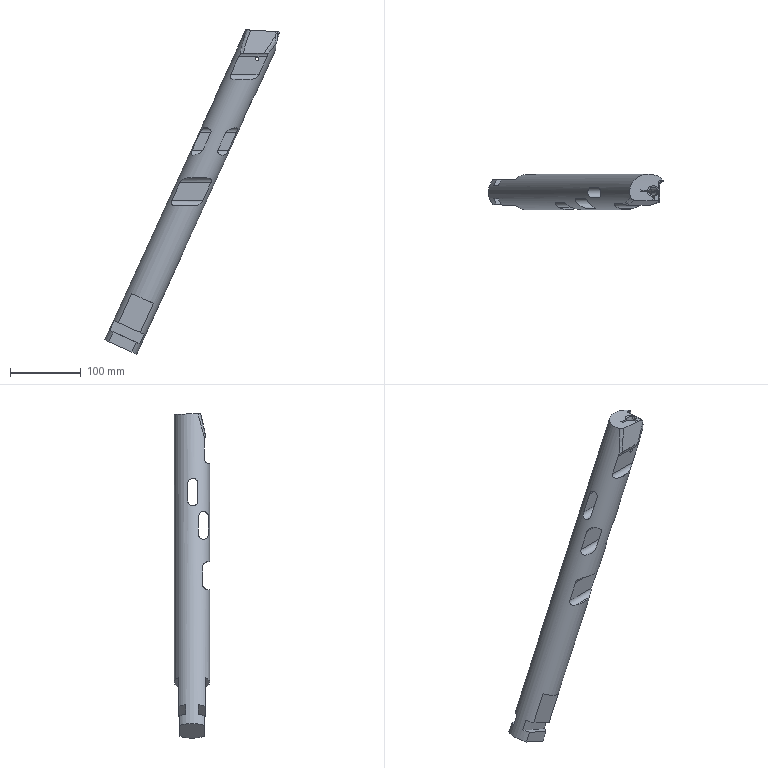Part | STEP file | solid 156 | 1 solid | 143 faces | box 247.177 x 50 x 457.681 mm | volume 843242 mm3 | plane 63 | other 46 | cylinder 15 | spline 14 | cone 3 | torus 2 | commonest cylinder face diameters 14 x8 5 x2 6 x2 4.02 x1 10 x1 50 x1